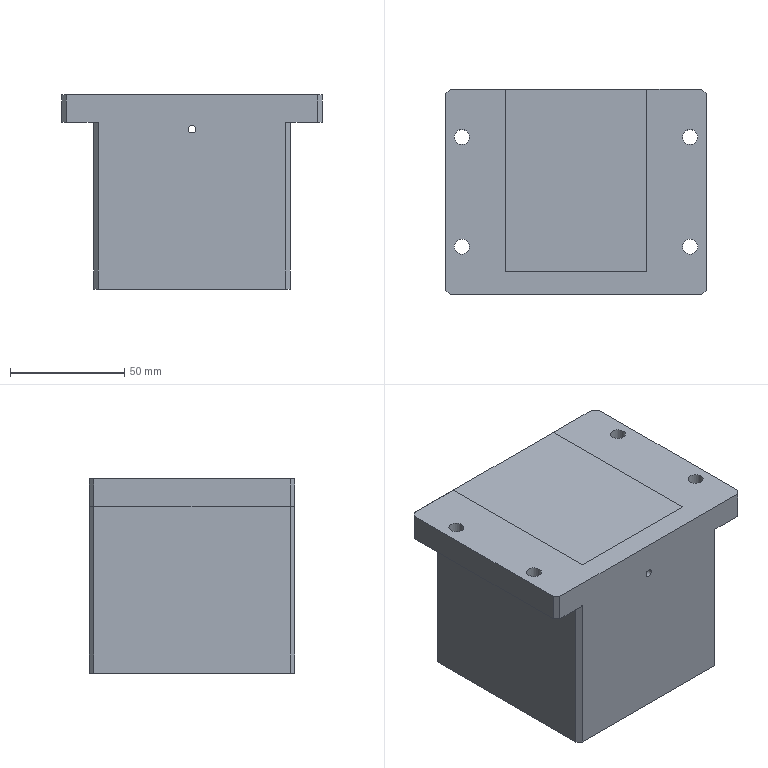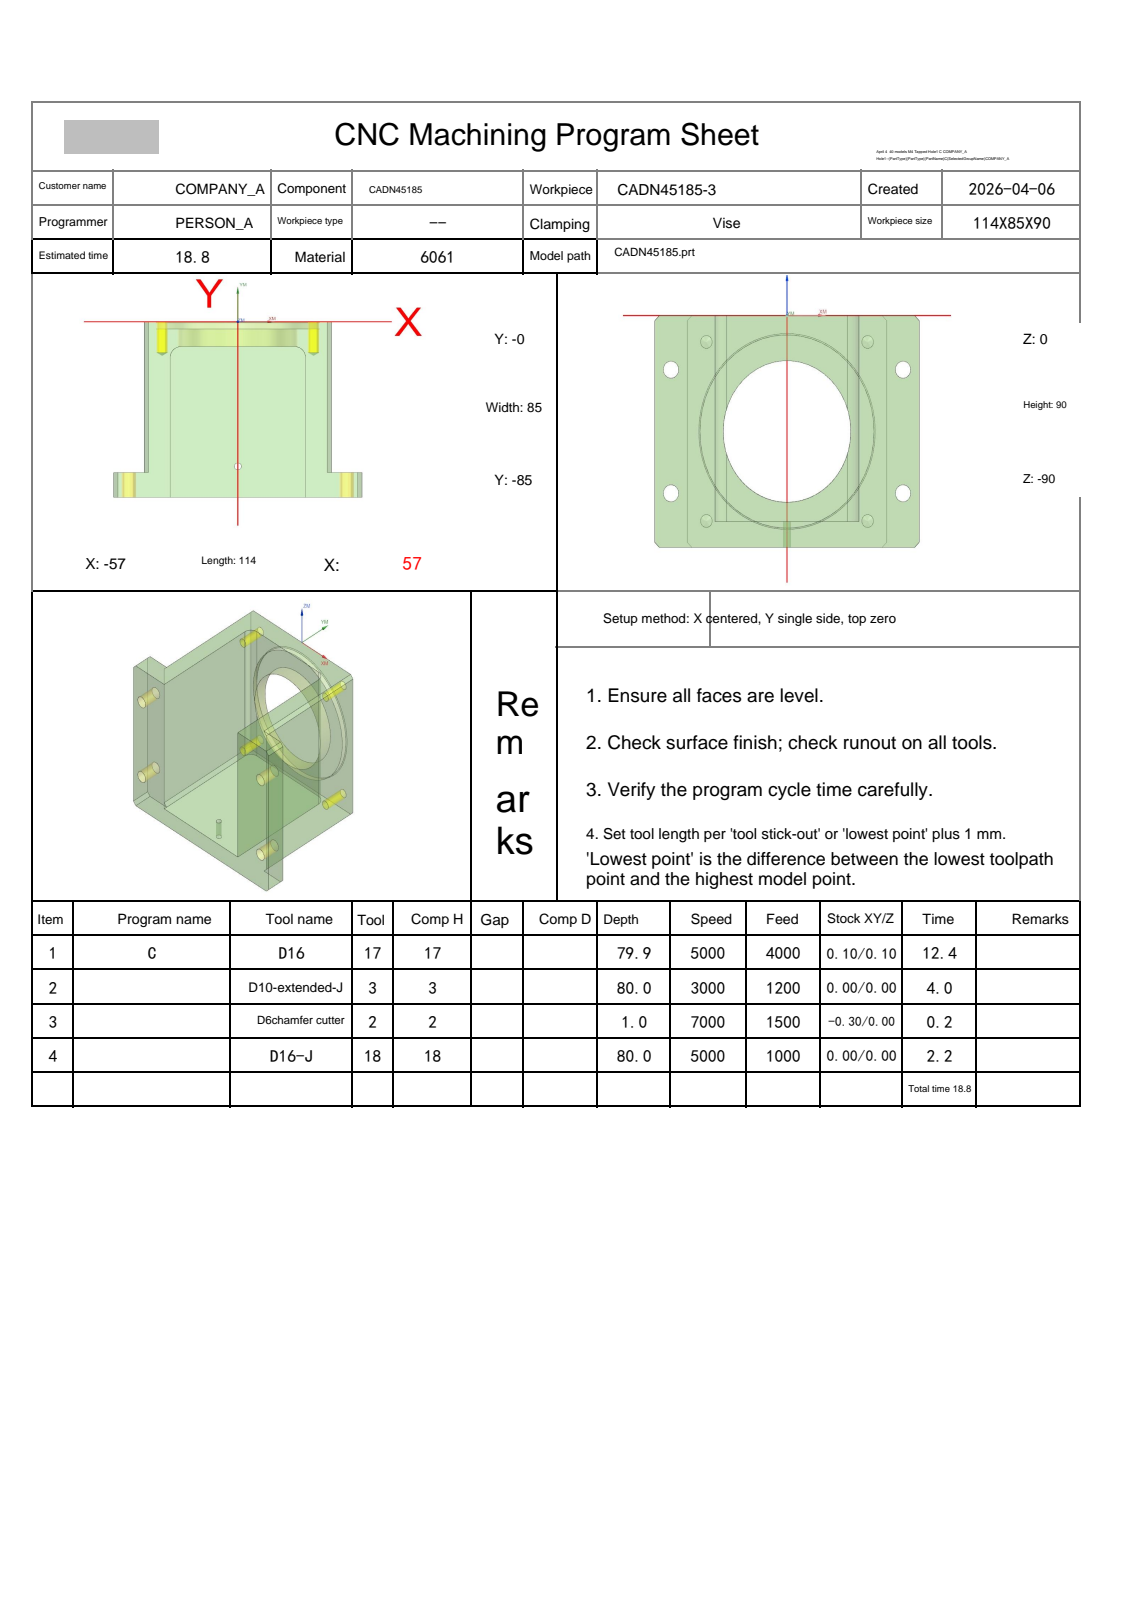NC program | NX | posted by the shop | part box 114 x 90 x 85 mm
Lines 1 to 1245 of 14367:
%
O0001
(Machine time: 19.44 MIN)
(===Total Tool:4===)
(T17=D16    D=16.  R=0.   D-  H17 Z=-79.9 )
(T3=D10-extended-J D=10.  R=0.   D-  H03 Z=-80.  )
(T2=D6chamfer cutter   D=6.   R=0.   D-  H02 Z=-1.   )
(T18=D16-J  D=16.  R=0.   D18 H18 Z=-80.  )
G80 G90 G17 G49 G40
G91 G28 Z0
M01
N1 T17 M06
(D16  D=16. R=0. H=17 ce=0.10 di=0.10)
G00 G90 G54 X3.936 Y-96. M03 S5000
G43 H17 Z10.1
M08
Z.701
G01 Z-.799 F4000.
X4.104 Y-92.84
X7.098 Y-36.478
G03 X7.104 Y-36.265 I-3.994 J.212
X3.104 Y-32.265 I-4. J0.0
X-.891 Y-36.053 I0.0 J-4.
G01 X-3.827 Y-91.325
G02 X-5.425 Y-92.84 I-1.598 J.085
G01 X-9.3
G02 X-10.9 Y-91.24 I0.0 J1.6
G01 Y-33.697
G02 X-9.303 Y-32.1 I1.6 J-.003
G01 X9.303
G02 X10.9 Y-33.697 I-.003 J-1.6
G01 Y-91.471
G03 X12.253 Y-93.051 I1.6 J.001
G01 X21.054 Y-94.421
G03 X21.3 Y-94.44 I.246 J1.581
X22.9 Y-92.84 I0.0 J1.6
G01 Y-20.1
X-22.9
Y-92.84
Y-96.1
Z.701
G00 X3.936 Y-96.
Z-.098
G01 Z-1.598
X4.104 Y-92.84
X7.098 Y-36.478
G03 X7.104 Y-36.265 I-3.994 J.212
X3.104 Y-32.265 I-4. J0.0
X-.891 Y-36.053 I0.0 J-4.
G01 X-3.827 Y-91.325
G02 X-5.425 Y-92.84 I-1.598 J.085
G01 X-9.3
G02 X-10.9 Y-91.24 I0.0 J1.6
G01 Y-33.697
G02 X-9.303 Y-32.1 I1.6 J-.003
G01 X9.303
G02 X10.9 Y-33.697 I-.003 J-1.6
G01 Y-91.471
G03 X12.253 Y-93.051 I1.6 J.001
G01 X21.054 Y-94.421
G03 X21.3 Y-94.44 I.246 J1.581
X22.9 Y-92.84 I0.0 J1.6
G01 Y-20.1
X-22.9
Y-92.84
Y-96.1
Z-.098
G00 X3.936 Y-96.
Z-.897
G01 Z-2.397
X4.104 Y-92.84
X7.098 Y-36.478
G03 X7.104 Y-36.265 I-3.994 J.212
X3.104 Y-32.265 I-4. J0.0
X-.891 Y-36.053 I0.0 J-4.
G01 X-3.827 Y-91.325
G02 X-5.425 Y-92.84 I-1.598 J.085
G01 X-9.3
G02 X-10.9 Y-91.24 I0.0 J1.6
G01 Y-33.697
G02 X-9.303 Y-32.1 I1.6 J-.003
G01 X9.303
G02 X10.9 Y-33.697 I-.003 J-1.6
G01 Y-91.471
G03 X12.253 Y-93.051 I1.6 J.001
G01 X21.054 Y-94.421
G03 X21.3 Y-94.44 I.246 J1.581
X22.9 Y-92.84 I0.0 J1.6
G01 Y-20.1
X-22.9
Y-92.84
Y-96.1
Z-.897
G00 X3.936 Y-96.
Z-1.696
G01 Z-3.196
X4.104 Y-92.84
X7.098 Y-36.478
G03 X7.104 Y-36.265 I-3.994 J.212
X3.104 Y-32.265 I-4. J0.0
X-.891 Y-36.053 I0.0 J-4.
G01 X-3.827 Y-91.325
G02 X-5.425 Y-92.84 I-1.598 J.085
G01 X-9.3
G02 X-10.9 Y-91.24 I0.0 J1.6
G01 Y-33.697
G02 X-9.303 Y-32.1 I1.6 J-.003
G01 X9.303
G02 X10.9 Y-33.697 I-.003 J-1.6
G01 Y-91.471
G03 X12.253 Y-93.051 I1.6 J.001
G01 X21.054 Y-94.421
G03 X21.3 Y-94.44 I.246 J1.581
X22.9 Y-92.84 I0.0 J1.6
G01 Y-20.1
X-22.9
Y-92.84
Y-96.1
Z-1.696
G00 X3.936 Y-96.
Z-2.495
G01 Z-3.995
X4.104 Y-92.84
X7.098 Y-36.478
G03 X7.104 Y-36.265 I-3.994 J.212
X3.104 Y-32.265 I-4. J0.0
X-.891 Y-36.053 I0.0 J-4.
G01 X-3.827 Y-91.325
G02 X-5.425 Y-92.84 I-1.598 J.085
G01 X-9.3
G02 X-10.9 Y-91.24 I0.0 J1.6
G01 Y-33.697
G02 X-9.303 Y-32.1 I1.6 J-.003
G01 X9.303
G02 X10.9 Y-33.697 I-.003 J-1.6
G01 Y-91.471
G03 X12.253 Y-93.051 I1.6 J.001
G01 X21.054 Y-94.421
G03 X21.3 Y-94.44 I.246 J1.581
X22.9 Y-92.84 I0.0 J1.6
G01 Y-20.1
X-22.9
Y-92.84
Y-96.1
Z-2.495
G00 X3.936 Y-96.
Z-3.294
G01 Z-4.794
X4.104 Y-92.84
X7.098 Y-36.478
G03 X7.104 Y-36.265 I-3.994 J.212
X3.104 Y-32.265 I-4. J0.0
X-.891 Y-36.053 I0.0 J-4.
G01 X-3.827 Y-91.325
G02 X-5.425 Y-92.84 I-1.598 J.085
G01 X-9.3
G02 X-10.9 Y-91.24 I0.0 J1.6
G01 Y-33.697
G02 X-9.303 Y-32.1 I1.6 J-.003
G01 X9.303
G02 X10.9 Y-33.697 I-.003 J-1.6
G01 Y-91.471
G03 X12.253 Y-93.051 I1.6 J.001
G01 X21.054 Y-94.421
G03 X21.3 Y-94.44 I.246 J1.581
X22.9 Y-92.84 I0.0 J1.6
G01 Y-20.1
X-22.9
Y-92.84
Y-96.1
Z-3.294
G00 X3.936 Y-96.
Z-4.093
G01 Z-5.593
X4.104 Y-92.84
X7.098 Y-36.478
G03 X7.104 Y-36.265 I-3.994 J.212
X3.104 Y-32.265 I-4. J0.0
X-.891 Y-36.053 I0.0 J-4.
G01 X-3.827 Y-91.325
G02 X-5.425 Y-92.84 I-1.598 J.085
G01 X-9.3
G02 X-10.9 Y-91.24 I0.0 J1.6
G01 Y-33.697
G02 X-9.303 Y-32.1 I1.6 J-.003
G01 X9.303
G02 X10.9 Y-33.697 I-.003 J-1.6
G01 Y-91.471
G03 X12.253 Y-93.051 I1.6 J.001
G01 X21.054 Y-94.421
G03 X21.3 Y-94.44 I.246 J1.581
X22.9 Y-92.84 I0.0 J1.6
G01 Y-20.1
X-22.9
Y-92.84
Y-96.1
Z-4.093
G00 X3.936 Y-96.
Z-4.892
G01 Z-6.392
X4.104 Y-92.84
X7.098 Y-36.478
G03 X7.104 Y-36.265 I-3.994 J.212
X3.104 Y-32.265 I-4. J0.0
X-.891 Y-36.053 I0.0 J-4.
G01 X-3.827 Y-91.325
G02 X-5.425 Y-92.84 I-1.598 J.085
G01 X-9.3
G02 X-10.9 Y-91.24 I0.0 J1.6
G01 Y-33.697
G02 X-9.303 Y-32.1 I1.6 J-.003
G01 X9.303
G02 X10.9 Y-33.697 I-.003 J-1.6
G01 Y-91.471
G03 X12.253 Y-93.051 I1.6 J.001
G01 X21.054 Y-94.421
G03 X21.3 Y-94.44 I.246 J1.581
X22.9 Y-92.84 I0.0 J1.6
G01 Y-20.1
X-22.9
Y-92.84
Y-96.1
Z-4.892
G00 X3.936 Y-96.
Z-5.691
G01 Z-7.191
X4.104 Y-92.84
X7.098 Y-36.478
G03 X7.104 Y-36.265 I-3.994 J.212
X3.104 Y-32.265 I-4. J0.0
X-.891 Y-36.053 I0.0 J-4.
G01 X-3.827 Y-91.325
G02 X-5.425 Y-92.84 I-1.598 J.085
G01 X-9.3
G02 X-10.9 Y-91.24 I0.0 J1.6
G01 Y-33.697
G02 X-9.303 Y-32.1 I1.6 J-.003
G01 X9.303
G02 X10.9 Y-33.697 I-.003 J-1.6
G01 Y-91.471
G03 X12.253 Y-93.051 I1.6 J.001
G01 X21.054 Y-94.421
G03 X21.3 Y-94.44 I.246 J1.581
X22.9 Y-92.84 I0.0 J1.6
G01 Y-20.1
X-22.9
Y-92.84
Y-96.1
Z-5.691
G00 X3.936 Y-96.
Z-6.49
G01 Z-7.99
X4.104 Y-92.84
X7.098 Y-36.478
G03 X7.104 Y-36.265 I-3.994 J.212
X3.104 Y-32.265 I-4. J0.0
X-.891 Y-36.053 I0.0 J-4.
G01 X-3.827 Y-91.325
G02 X-5.425 Y-92.84 I-1.598 J.085
G01 X-9.3
G02 X-10.9 Y-91.24 I0.0 J1.6
G01 Y-33.697
G02 X-9.303 Y-32.1 I1.6 J-.003
G01 X9.303
G02 X10.9 Y-33.697 I-.003 J-1.6
G01 Y-91.471
G03 X12.253 Y-93.051 I1.6 J.001
G01 X21.054 Y-94.421
G03 X21.3 Y-94.44 I.246 J1.581
X22.9 Y-92.84 I0.0 J1.6
G01 Y-20.1
X-22.9
Y-92.84
Y-96.1
Z-6.49
G00 X3.936 Y-96.
Z-7.289
G01 Z-8.789
X4.104 Y-92.84
X7.098 Y-36.478
G03 X7.104 Y-36.265 I-3.994 J.212
X3.104 Y-32.265 I-4. J0.0
X-.891 Y-36.053 I0.0 J-4.
G01 X-3.827 Y-91.325
G02 X-5.425 Y-92.84 I-1.598 J.085
G01 X-9.3
G02 X-10.9 Y-91.24 I0.0 J1.6
G01 Y-33.697
G02 X-9.303 Y-32.1 I1.6 J-.003
G01 X9.303
G02 X10.9 Y-33.697 I-.003 J-1.6
G01 Y-91.471
G03 X12.253 Y-93.051 I1.6 J.001
G01 X21.054 Y-94.421
G03 X21.3 Y-94.44 I.246 J1.581
X22.9 Y-92.84 I0.0 J1.6
G01 Y-20.1
X-22.9
Y-92.84
Y-96.1
Z-7.289
G00 X3.936 Y-96.
Z-8.088
G01 Z-9.588
X4.104 Y-92.84
X7.098 Y-36.478
G03 X7.104 Y-36.265 I-3.994 J.212
X3.104 Y-32.265 I-4. J0.0
X-.891 Y-36.053 I0.0 J-4.
G01 X-3.827 Y-91.325
G02 X-5.425 Y-92.84 I-1.598 J.085
G01 X-9.3
G02 X-10.9 Y-91.24 I0.0 J1.6
G01 Y-33.697
G02 X-9.303 Y-32.1 I1.6 J-.003
G01 X9.303
G02 X10.9 Y-33.697 I-.003 J-1.6
G01 Y-91.471
G03 X12.253 Y-93.051 I1.6 J.001
G01 X21.054 Y-94.421
G03 X21.3 Y-94.44 I.246 J1.581
X22.9 Y-92.84 I0.0 J1.6
G01 Y-20.1
X-22.9
Y-92.84
Y-96.1
Z-8.088
G00 X3.936 Y-96.
Z-8.887
G01 Z-10.387
X4.104 Y-92.84
X7.098 Y-36.478
G03 X7.104 Y-36.265 I-3.994 J.212
X3.104 Y-32.265 I-4. J0.0
X-.891 Y-36.053 I0.0 J-4.
G01 X-3.827 Y-91.325
G02 X-5.425 Y-92.84 I-1.598 J.085
G01 X-9.3
G02 X-10.9 Y-91.24 I0.0 J1.6
G01 Y-33.697
G02 X-9.303 Y-32.1 I1.6 J-.003
G01 X9.303
G02 X10.9 Y-33.697 I-.003 J-1.6
G01 Y-91.471
G03 X12.253 Y-93.051 I1.6 J.001
G01 X21.054 Y-94.421
G03 X21.3 Y-94.44 I.246 J1.581
X22.9 Y-92.84 I0.0 J1.6
G01 Y-20.1
X-22.9
Y-92.84
Y-96.1
Z-8.887
G00 X3.936 Y-96.
Z-9.686
G01 Z-11.186
X4.104 Y-92.84
X7.098 Y-36.478
G03 X7.104 Y-36.265 I-3.994 J.212
X3.104 Y-32.265 I-4. J0.0
X-.891 Y-36.053 I0.0 J-4.
G01 X-3.827 Y-91.325
G02 X-5.425 Y-92.84 I-1.598 J.085
G01 X-9.3
G02 X-10.9 Y-91.24 I0.0 J1.6
G01 Y-33.697
G02 X-9.303 Y-32.1 I1.6 J-.003
G01 X9.303
G02 X10.9 Y-33.697 I-.003 J-1.6
G01 Y-91.471
G03 X12.253 Y-93.051 I1.6 J.001
G01 X21.054 Y-94.421
G03 X21.3 Y-94.44 I.246 J1.581
X22.9 Y-92.84 I0.0 J1.6
G01 Y-20.1
X-22.9
Y-92.84
Y-96.1
Z-9.686
G00 X3.936 Y-96.
Z-10.485
G01 Z-11.985
X4.104 Y-92.84
X7.098 Y-36.478
G03 X7.104 Y-36.265 I-3.994 J.212
X3.104 Y-32.265 I-4. J0.0
X-.891 Y-36.053 I0.0 J-4.
G01 X-3.827 Y-91.325
G02 X-5.425 Y-92.84 I-1.598 J.085
G01 X-9.3
G02 X-10.9 Y-91.24 I0.0 J1.6
G01 Y-33.697
G02 X-9.303 Y-32.1 I1.6 J-.003
G01 X9.303
G02 X10.9 Y-33.697 I-.003 J-1.6
G01 Y-91.471
G03 X12.253 Y-93.051 I1.6 J.001
G01 X21.054 Y-94.421
G03 X21.3 Y-94.44 I.246 J1.581
X22.9 Y-92.84 I0.0 J1.6
G01 Y-20.1
X-22.9
Y-92.84
Y-96.1
Z-10.485
G00 X3.936 Y-96.
Z-11.284
G01 Z-12.784
X4.104 Y-92.84
X7.098 Y-36.478
G03 X7.104 Y-36.265 I-3.994 J.212
X3.104 Y-32.265 I-4. J0.0
X-.891 Y-36.053 I0.0 J-4.
G01 X-3.827 Y-91.325
G02 X-5.425 Y-92.84 I-1.598 J.085
G01 X-9.3
G02 X-10.9 Y-91.24 I0.0 J1.6
G01 Y-33.697
G02 X-9.303 Y-32.1 I1.6 J-.003
G01 X9.303
G02 X10.9 Y-33.697 I-.003 J-1.6
G01 Y-91.471
G03 X12.253 Y-93.051 I1.6 J.001
G01 X21.054 Y-94.421
G03 X21.3 Y-94.44 I.246 J1.581
X22.9 Y-92.84 I0.0 J1.6
G01 Y-20.1
X-22.9
Y-92.84
Y-96.1
Z-11.284
G00 X3.936 Y-96.
Z-12.083
G01 Z-13.583
X4.104 Y-92.84
X7.098 Y-36.478
G03 X7.104 Y-36.265 I-3.994 J.212
X3.104 Y-32.265 I-4. J0.0
X-.891 Y-36.053 I0.0 J-4.
G01 X-3.827 Y-91.325
G02 X-5.425 Y-92.84 I-1.598 J.085
G01 X-9.3
G02 X-10.9 Y-91.24 I0.0 J1.6
G01 Y-33.697
G02 X-9.303 Y-32.1 I1.6 J-.003
G01 X9.303
G02 X10.9 Y-33.697 I-.003 J-1.6
G01 Y-91.471
G03 X12.253 Y-93.051 I1.6 J.001
G01 X21.054 Y-94.421
G03 X21.3 Y-94.44 I.246 J1.581
X22.9 Y-92.84 I0.0 J1.6
G01 Y-20.1
X-22.9
Y-92.84
Y-96.1
Z-12.083
G00 X3.936 Y-96.
Z-12.882
G01 Z-14.382
X4.104 Y-92.84
X7.098 Y-36.478
G03 X7.104 Y-36.265 I-3.994 J.212
X3.104 Y-32.265 I-4. J0.0
X-.891 Y-36.053 I0.0 J-4.
G01 X-3.827 Y-91.325
G02 X-5.425 Y-92.84 I-1.598 J.085
G01 X-9.3
G02 X-10.9 Y-91.24 I0.0 J1.6
G01 Y-33.697
G02 X-9.303 Y-32.1 I1.6 J-.003
G01 X9.303
G02 X10.9 Y-33.697 I-.003 J-1.6
G01 Y-91.471
G03 X12.253 Y-93.051 I1.6 J.001
G01 X21.054 Y-94.421
G03 X21.3 Y-94.44 I.246 J1.581
X22.9 Y-92.84 I0.0 J1.6
G01 Y-20.1
X-22.9
Y-92.84
Y-96.1
Z-12.882
G00 X3.936 Y-96.
Z-13.681
G01 Z-15.181
X4.104 Y-92.84
X7.098 Y-36.478
G03 X7.104 Y-36.265 I-3.994 J.212
X3.104 Y-32.265 I-4. J0.0
X-.891 Y-36.053 I0.0 J-4.
G01 X-3.827 Y-91.325
G02 X-5.425 Y-92.84 I-1.598 J.085
G01 X-9.3
G02 X-10.9 Y-91.24 I0.0 J1.6
G01 Y-33.697
G02 X-9.303 Y-32.1 I1.6 J-.003
G01 X9.303
G02 X10.9 Y-33.697 I-.003 J-1.6
G01 Y-91.471
G03 X12.253 Y-93.051 I1.6 J.001
G01 X21.054 Y-94.421
G03 X21.3 Y-94.44 I.246 J1.581
X22.9 Y-92.84 I0.0 J1.6
G01 Y-20.1
X-22.9
Y-92.84
Y-96.1
Z-13.681
G00 X3.936 Y-96.
Z-14.48
G01 Z-15.98
X4.104 Y-92.84
X7.098 Y-36.478
G03 X7.104 Y-36.265 I-3.994 J.212
X3.104 Y-32.265 I-4. J0.0
X-.891 Y-36.053 I0.0 J-4.
G01 X-3.827 Y-91.325
G02 X-5.425 Y-92.84 I-1.598 J.085
G01 X-9.3
G02 X-10.9 Y-91.24 I0.0 J1.6
G01 Y-33.697
G02 X-9.303 Y-32.1 I1.6 J-.003
G01 X9.303
G02 X10.9 Y-33.697 I-.003 J-1.6
G01 Y-91.471
G03 X12.253 Y-93.051 I1.6 J.001
G01 X21.054 Y-94.421
G03 X21.3 Y-94.44 I.246 J1.581
X22.9 Y-92.84 I0.0 J1.6
G01 Y-20.1
X-22.9
Y-92.84
Y-96.1
Z-14.48
G00 X3.936 Y-96.
Z-15.279
G01 Z-16.779
X4.104 Y-92.84
X7.098 Y-36.478
G03 X7.104 Y-36.265 I-3.994 J.212
X3.104 Y-32.265 I-4. J0.0
X-.891 Y-36.053 I0.0 J-4.
G01 X-3.827 Y-91.325
G02 X-5.425 Y-92.84 I-1.598 J.085
G01 X-9.3
G02 X-10.9 Y-91.24 I0.0 J1.6
G01 Y-33.697
G02 X-9.303 Y-32.1 I1.6 J-.003
G01 X9.303
G02 X10.9 Y-33.697 I-.003 J-1.6
G01 Y-91.471
G03 X12.253 Y-93.051 I1.6 J.001
G01 X21.054 Y-94.421
G03 X21.3 Y-94.44 I.246 J1.581
X22.9 Y-92.84 I0.0 J1.6
G01 Y-20.1
X-22.9
Y-92.84
Y-96.1
Z-15.279
G00 X3.936 Y-96.
Z-16.078
G01 Z-17.578
X4.104 Y-92.84
X7.098 Y-36.478
G03 X7.104 Y-36.265 I-3.994 J.212
X3.104 Y-32.265 I-4. J0.0
X-.891 Y-36.053 I0.0 J-4.
G01 X-3.827 Y-91.325
G02 X-5.425 Y-92.84 I-1.598 J.085
G01 X-9.3
G02 X-10.9 Y-91.24 I0.0 J1.6
G01 Y-33.697
G02 X-9.303 Y-32.1 I1.6 J-.003
G01 X9.303
G02 X10.9 Y-33.697 I-.003 J-1.6
G01 Y-91.471
G03 X12.253 Y-93.051 I1.6 J.001
G01 X21.054 Y-94.421
G03 X21.3 Y-94.44 I.246 J1.581
X22.9 Y-92.84 I0.0 J1.6
G01 Y-20.1
X-22.9
Y-92.84
Y-96.1
Z-16.078
G00 X3.936 Y-96.
Z-16.877
G01 Z-18.377
X4.104 Y-92.84
X7.098 Y-36.478
G03 X7.104 Y-36.265 I-3.994 J.212
X3.104 Y-32.265 I-4. J0.0
X-.891 Y-36.053 I0.0 J-4.
G01 X-3.827 Y-91.325
G02 X-5.425 Y-92.84 I-1.598 J.085
G01 X-9.3
G02 X-10.9 Y-91.24 I0.0 J1.6
G01 Y-33.697
G02 X-9.303 Y-32.1 I1.6 J-.003
G01 X9.303
G02 X10.9 Y-33.697 I-.003 J-1.6
G01 Y-91.471
G03 X12.253 Y-93.051 I1.6 J.001
G01 X21.054 Y-94.421
G03 X21.3 Y-94.44 I.246 J1.581
X22.9 Y-92.84 I0.0 J1.6
G01 Y-20.1
X-22.9
Y-92.84
Y-96.1
Z-16.877
G00 X3.936 Y-96.
Z-17.676
G01 Z-19.176
X4.104 Y-92.84
X7.098 Y-36.478
G03 X7.104 Y-36.265 I-3.994 J.212
X3.104 Y-32.265 I-4. J0.0
X-.891 Y-36.053 I0.0 J-4.
G01 X-3.827 Y-91.325
G02 X-5.425 Y-92.84 I-1.598 J.085
G01 X-9.3
G02 X-10.9 Y-91.24 I0.0 J1.6
G01 Y-33.697
G02 X-9.303 Y-32.1 I1.6 J-.003
G01 X9.303
G02 X10.9 Y-33.697 I-.003 J-1.6
G01 Y-91.471
G03 X12.253 Y-93.051 I1.6 J.001
G01 X21.054 Y-94.421
G03 X21.3 Y-94.44 I.246 J1.581
X22.9 Y-92.84 I0.0 J1.6
G01 Y-20.1
X-22.9
Y-92.84
Y-96.1
Z-17.676
G00 X3.936 Y-96.
Z-18.475
G01 Z-19.975
X4.104 Y-92.84
X7.098 Y-36.478
G03 X7.104 Y-36.265 I-3.994 J.212
X3.104 Y-32.265 I-4. J0.0
X-.891 Y-36.053 I0.0 J-4.
G01 X-3.827 Y-91.325
G02 X-5.425 Y-92.84 I-1.598 J.085
G01 X-9.3
G02 X-10.9 Y-91.24 I0.0 J1.6
G01 Y-33.697
G02 X-9.303 Y-32.1 I1.6 J-.003
G01 X9.303
G02 X10.9 Y-33.697 I-.003 J-1.6
G01 Y-91.471
G03 X12.253 Y-93.051 I1.6 J.001
G01 X21.054 Y-94.421
G03 X21.3 Y-94.44 I.246 J1.581
X22.9 Y-92.84 I0.0 J1.6
G01 Y-20.1
X-22.9
Y-92.84
Y-96.1
Z-18.475
G00 X3.936 Y-96.
Z-19.274
G01 Z-20.774
X4.104 Y-92.84
X7.098 Y-36.478
G03 X7.104 Y-36.265 I-3.994 J.212
X3.104 Y-32.265 I-4. J0.0
X-.891 Y-36.053 I0.0 J-4.
G01 X-3.827 Y-91.325
G02 X-5.425 Y-92.84 I-1.598 J.085
G01 X-9.3
G02 X-10.9 Y-91.24 I0.0 J1.6
G01 Y-33.697
G02 X-9.303 Y-32.1 I1.6 J-.003
G01 X9.303
G02 X10.9 Y-33.697 I-.003 J-1.6
G01 Y-91.471
G03 X12.253 Y-93.051 I1.6 J.001
G01 X21.054 Y-94.421
G03 X21.3 Y-94.44 I.246 J1.581
X22.9 Y-92.84 I0.0 J1.6
G01 Y-20.1
X-22.9
Y-92.84
Y-96.1
Z-19.274
G00 X3.936 Y-96.
Z-20.073
G01 Z-21.573
X4.104 Y-92.84
X7.098 Y-36.478
G03 X7.104 Y-36.265 I-3.994 J.212
X3.104 Y-32.265 I-4. J0.0
X-.891 Y-36.053 I0.0 J-4.
G01 X-3.827 Y-91.325
G02 X-5.425 Y-92.84 I-1.598 J.085
G01 X-9.3
G02 X-10.9 Y-91.24 I0.0 J1.6
G01 Y-33.697
G02 X-9.303 Y-32.1 I1.6 J-.003
G01 X9.303
G02 X10.9 Y-33.697 I-.003 J-1.6
G01 Y-91.471
G03 X12.253 Y-93.051 I1.6 J.001
G01 X21.054 Y-94.421
G03 X21.3 Y-94.44 I.246 J1.581
X22.9 Y-92.84 I0.0 J1.6
G01 Y-20.1
X-22.9
Y-92.84
Y-96.1
Z-20.073
G00 X3.936 Y-96.
Z-20.872
G01 Z-22.372
X4.104 Y-92.84
X7.098 Y-36.478
G03 X7.104 Y-36.265 I-3.994 J.212
X3.104 Y-32.265 I-4. J0.0
X-.891 Y-36.053 I0.0 J-4.
G01 X-3.827 Y-91.325
G02 X-5.425 Y-92.84 I-1.598 J.085
G01 X-9.3
G02 X-10.9 Y-91.24 I0.0 J1.6
G01 Y-33.697
G02 X-9.303 Y-32.1 I1.6 J-.003
G01 X9.303
G02 X10.9 Y-33.697 I-.003 J-1.6
G01 Y-91.471
G03 X12.253 Y-93.051 I1.6 J.001
G01 X21.054 Y-94.421
G03 X21.3 Y-94.44 I.246 J1.581
X22.9 Y-92.84 I0.0 J1.6
G01 Y-20.1
X-22.9
Y-92.84
Y-96.1
Z-20.872
G00 X3.936 Y-96.
Z-21.671
G01 Z-23.171
X4.104 Y-92.84
X7.098 Y-36.478
G03 X7.104 Y-36.265 I-3.994 J.212
X3.104 Y-32.265 I-4. J0.0
X-.891 Y-36.053 I0.0 J-4.
G01 X-3.827 Y-91.325
G02 X-5.425 Y-92.84 I-1.598 J.085
G01 X-9.3
G02 X-10.9 Y-91.24 I0.0 J1.6
G01 Y-33.697
G02 X-9.303 Y-32.1 I1.6 J-.003
G01 X9.303
G02 X10.9 Y-33.697 I-.003 J-1.6
G01 Y-91.471
G03 X12.253 Y-93.051 I1.6 J.001
G01 X21.054 Y-94.421
G03 X21.3 Y-94.44 I.246 J1.581
X22.9 Y-92.84 I0.0 J1.6
G01 Y-20.1
X-22.9
Y-92.84
Y-96.1
Z-21.671
G00 X3.936 Y-96.
Z-22.47
G01 Z-23.97
X4.104 Y-92.84
X7.098 Y-36.478
G03 X7.104 Y-36.265 I-3.994 J.212
X3.104 Y-32.265 I-4. J0.0
X-.891 Y-36.053 I0.0 J-4.
G01 X-3.827 Y-91.325
G02 X-5.425 Y-92.84 I-1.598 J.085
G01 X-9.3
G02 X-10.9 Y-91.24 I0.0 J1.6
G01 Y-33.697
G02 X-9.303 Y-32.1 I1.6 J-.003
G01 X9.303
G02 X10.9 Y-33.697 I-.003 J-1.6
G01 Y-91.471
G03 X12.253 Y-93.051 I1.6 J.001
G01 X21.054 Y-94.421
G03 X21.3 Y-94.44 I.246 J1.581
X22.9 Y-92.84 I0.0 J1.6
G01 Y-20.1
X-22.9
Y-92.84
Y-96.1
Z-22.47
G00 X3.936 Y-96.
Z-23.269
G01 Z-24.769
X4.104 Y-92.84
X7.098 Y-36.478
G03 X7.104 Y-36.265 I-3.994 J.212
X3.104 Y-32.265 I-4. J0.0
X-.891 Y-36.053 I0.0 J-4.
G01 X-3.827 Y-91.325
G02 X-5.425 Y-92.84 I-1.598 J.085
G01 X-9.3
G02 X-10.9 Y-91.24 I0.0 J1.6
G01 Y-33.697
G02 X-9.303 Y-32.1 I1.6 J-.003
G01 X9.303
G02 X10.9 Y-33.697 I-.003 J-1.6
G01 Y-91.471
G03 X12.253 Y-93.051 I1.6 J.001
G01 X21.054 Y-94.421
G03 X21.3 Y-94.44 I.246 J1.581
X22.9 Y-92.84 I0.0 J1.6
G01 Y-20.1
X-22.9
Y-92.84
Y-96.1
Z-23.269
G00 X3.936 Y-96.
Z-24.068
G01 Z-25.568
X4.104 Y-92.84
X7.098 Y-36.478
G03 X7.104 Y-36.265 I-3.994 J.212
X3.104 Y-32.265 I-4. J0.0
X-.891 Y-36.053 I0.0 J-4.
G01 X-3.827 Y-91.325
G02 X-5.425 Y-92.84 I-1.598 J.085
G01 X-9.3
G02 X-10.9 Y-91.24 I0.0 J1.6
G01 Y-33.697
G02 X-9.303 Y-32.1 I1.6 J-.003
G01 X9.303
G02 X10.9 Y-33.697 I-.003 J-1.6
G01 Y-91.471
G03 X12.253 Y-93.051 I1.6 J.001
G01 X21.054 Y-94.421
G03 X21.3 Y-94.44 I.246 J1.581
X22.9 Y-92.84 I0.0 J1.6
G01 Y-20.1
X-22.9
Y-92.84
Y-96.1
Z-24.068
G00 X3.936 Y-96.
Z-24.867
G01 Z-26.367
X4.104 Y-92.84
X7.098 Y-36.478
G03 X7.104 Y-36.265 I-3.994 J.212
X3.104 Y-32.265 I-4. J0.0
X-.891 Y-36.053 I0.0 J-4.
G01 X-3.827 Y-91.325
G02 X-5.425 Y-92.84 I-1.598 J.085
G01 X-9.3
G02 X-10.9 Y-91.24 I0.0 J1.6
G01 Y-33.697
G02 X-9.303 Y-32.1 I1.6 J-.003
G01 X9.303
G02 X10.9 Y-33.697 I-.003 J-1.6
G01 Y-91.471
G03 X12.253 Y-93.051 I1.6 J.001
G01 X21.054 Y-94.421
G03 X21.3 Y-94.44 I.246 J1.581
X22.9 Y-92.84 I0.0 J1.6
G01 Y-20.1
X-22.9
Y-92.84
Y-96.1
Z-24.867
G00 X3.936 Y-96.
Z-25.666
G01 Z-27.166
X4.104 Y-92.84
X7.098 Y-36.478
G03 X7.104 Y-36.265 I-3.994 J.212
X3.104 Y-32.265 I-4. J0.0
X-.891 Y-36.053 I0.0 J-4.
G01 X-3.827 Y-91.325
G02 X-5.425 Y-92.84 I-1.598 J.085
G01 X-9.3
G02 X-10.9 Y-91.24 I0.0 J1.6
G01 Y-33.697
G02 X-9.303 Y-32.1 I1.6 J-.003
G01 X9.303
G02 X10.9 Y-33.697 I-.003 J-1.6
G01 Y-91.471
G03 X12.253 Y-93.051 I1.6 J.001
G01 X21.054 Y-94.421
G03 X21.3 Y-94.44 I.246 J1.581
X22.9 Y-92.84 I0.0 J1.6
G01 Y-20.1
X-22.9
Y-92.84
Y-96.1
Z-25.666
G00 X3.936 Y-96.
Z-26.465
G01 Z-27.965
X4.104 Y-92.84
X7.098 Y-36.478
G03 X7.104 Y-36.265 I-3.994 J.212
X3.104 Y-32.265 I-4. J0.0
X-.891 Y-36.053 I0.0 J-4.
G01 X-3.827 Y-91.325
G02 X-5.425 Y-92.84 I-1.598 J.085
G01 X-9.3
G02 X-10.9 Y-91.24 I0.0 J1.6
G01 Y-33.697
G02 X-9.303 Y-32.1 I1.6 J-.003
G01 X9.303
G02 X10.9 Y-33.697 I-.003 J-1.6
G01 Y-91.471
G03 X12.253 Y-93.051 I1.6 J.001
G01 X21.054 Y-94.421
G03 X21.3 Y-94.44 I.246 J1.581
X22.9 Y-92.84 I0.0 J1.6
G01 Y-20.1
X-22.9
Y-92.84
Y-96.1
Z-26.465
G00 X3.936 Y-96.
Z-27.264
G01 Z-28.764
X4.104 Y-92.84
X7.098 Y-36.478
G03 X7.104 Y-36.265 I-3.994 J.212
X3.104 Y-32.265 I-4. J0.0
X-.891 Y-36.053 I0.0 J-4.
G01 X-3.827 Y-91.325
G02 X-5.425 Y-92.84 I-1.598 J.085
G01 X-9.3
G02 X-10.9 Y-91.24 I0.0 J1.6
G01 Y-33.697
G02 X-9.303 Y-32.1 I1.6 J-.003
G01 X9.303
G02 X10.9 Y-33.697 I-.003 J-1.6
G01 Y-91.471
G03 X12.253 Y-93.051 I1.6 J.001
G01 X21.054 Y-94.421
G03 X21.3 Y-94.44 I.246 J1.581
X22.9 Y-92.84 I0.0 J1.6
G01 Y-20.1
X-22.9
Y-92.84
Y-96.1
Z-27.264
G00 X3.936 Y-96.
Z-28.063
G01 Z-29.563
X4.104 Y-92.84
X7.098 Y-36.478
G03 X7.104 Y-36.265 I-3.994 J.212
X3.104 Y-32.265 I-4. J0.0
X-.891 Y-36.053 I0.0 J-4.
G01 X-3.827 Y-91.325
G02 X-5.425 Y-92.84 I-1.598 J.085
G01 X-9.3
G02 X-10.9 Y-91.24 I0.0 J1.6
G01 Y-33.697
G02 X-9.303 Y-32.1 I1.6 J-.003
G01 X9.303
G02 X10.9 Y-33.697 I-.003 J-1.6
G01 Y-91.471
G03 X12.253 Y-93.051 I1.6 J.001
G01 X21.054 Y-94.421
G03 X21.3 Y-94.44 I.246 J1.581
X22.9 Y-92.84 I0.0 J1.6
G01 Y-20.1
X-22.9
Y-92.84
Y-96.1
Z-28.063
G00 X3.936 Y-96.
Z-28.862
G01 Z-30.362
X4.104 Y-92.84
X7.098 Y-36.478
G03 X7.104 Y-36.265 I-3.994 J.212
X3.104 Y-32.265 I-4. J0.0
X-.891 Y-36.053 I0.0 J-4.
G01 X-3.827 Y-91.325
G02 X-5.425 Y-92.84 I-1.598 J.085
G01 X-9.3
G02 X-10.9 Y-91.24 I0.0 J1.6
G01 Y-33.697
G02 X-9.303 Y-32.1 I1.6 J-.003
G01 X9.303
G02 X10.9 Y-33.697 I-.003 J-1.6
G01 Y-91.471
G03 X12.253 Y-93.051 I1.6 J.001
G01 X21.054 Y-94.421
G03 X21.3 Y-94.44 I.246 J1.581
X22.9 Y-92.84 I0.0 J1.6
G01 Y-20.1
X-22.9
Y-92.84
Y-96.1
Z-28.862
G00 X3.936 Y-96.
Z-29.661
G01 Z-31.161
X4.104 Y-92.84
X7.098 Y-36.478
G03 X7.104 Y-36.265 I-3.994 J.212
X3.104 Y-32.265 I-4. J0.0
X-.891 Y-36.053 I0.0 J-4.
G01 X-3.827 Y-91.325
G02 X-5.425 Y-92.84 I-1.598 J.085
G01 X-9.3
G02 X-10.9 Y-91.24 I0.0 J1.6
G01 Y-33.697
G02 X-9.303 Y-32.1 I1.6 J-.003
G01 X9.303
G02 X10.9 Y-33.697 I-.003 J-1.6
G01 Y-91.471
G03 X12.253 Y-93.051 I1.6 J.001
G01 X21.054 Y-94.421
G03 X21.3 Y-94.44 I.246 J1.581
X22.9 Y-92.84 I0.0 J1.6
G01 Y-20.1
X-22.9
Y-92.84
Y-96.1
Z-29.661
G00 X3.936 Y-96.
Z-30.46
G01 Z-31.96
X4.104 Y-92.84
X7.098 Y-36.478
G03 X7.104 Y-36.265 I-3.994 J.212
X3.104 Y-32.265 I-4. J0.0
X-.891 Y-36.053 I0.0 J-4.
G01 X-3.827 Y-91.325
G02 X-5.425 Y-92.84 I-1.598 J.085
G01 X-9.3
G02 X-10.9 Y-91.24 I0.0 J1.6
G01 Y-33.697
G02 X-9.303 Y-32.1 I1.6 J-.003
G01 X9.303
G02 X10.9 Y-33.697 I-.003 J-1.6
G01 Y-91.471
G03 X12.253 Y-93.051 I1.6 J.001
G01 X21.054 Y-94.421
G03 X21.3 Y-94.44 I.246 J1.581
X22.9 Y-92.84 I0.0 J1.6
G01 Y-20.1
X-22.9
Y-92.84
Y-96.1
Z-30.46
G00 X3.936 Y-96.
Z-31.259
G01 Z-32.759
X4.104 Y-92.84
X7.098 Y-36.478
G03 X7.104 Y-36.265 I-3.994 J.212
X3.104 Y-32.265 I-4. J0.0
X-.891 Y-36.053 I0.0 J-4.
G01 X-3.827 Y-91.325
G02 X-5.425 Y-92.84 I-1.598 J.085
G01 X-9.3
G02 X-10.9 Y-91.24 I0.0 J1.6
G01 Y-33.697
G02 X-9.303 Y-32.1 I1.6 J-.003
G01 X9.303
G02 X10.9 Y-33.697 I-.003 J-1.6
G01 Y-91.471
G03 X12.253 Y-93.051 I1.6 J.001
G01 X21.054 Y-94.421
G03 X21.3 Y-94.44 I.246 J1.581
X22.9 Y-92.84 I0.0 J1.6
G01 Y-20.1
X-22.9
Y-92.84
Y-96.1
Z-31.259
G00 X3.936 Y-96.
Z-32.058
G01 Z-33.558
X4.104 Y-92.84
X7.098 Y-36.478
G03 X7.104 Y-36.265 I-3.994 J.212
X3.104 Y-32.265 I-4. J0.0
X-.891 Y-36.053 I0.0 J-4.
G01 X-3.827 Y-91.325
G02 X-5.425 Y-92.84 I-1.598 J.085
G01 X-9.3
G02 X-10.9 Y-91.24 I0.0 J1.6
G01 Y-33.697
G02 X-9.303 Y-32.1 I1.6 J-.003
G01 X9.303
G02 X10.9 Y-33.697 I-.003 J-1.6
G01 Y-91.471
G03 X12.253 Y-93.051 I1.6 J.001
G01 X21.054 Y-94.421
G03 X21.3 Y-94.44 I.246 J1.581
X22.9 Y-92.84 I0.0 J1.6
G01 Y-20.1
X-22.9
Y-92.84
Y-96.1
Z-32.058
G00 X3.936 Y-96.
Z-32.857
G01 Z-34.357
X4.104 Y-92.84
X7.098 Y-36.478
G03 X7.104 Y-36.265 I-3.994 J.212
X3.104 Y-32.265 I-4. J0.0
X-.891 Y-36.053 I0.0 J-4.
G01 X-3.827 Y-91.325
G02 X-5.425 Y-92.84 I-1.598 J.085
G01 X-9.3
G02 X-10.9 Y-91.24 I0.0 J1.6
G01 Y-33.697
G02 X-9.303 Y-32.1 I1.6 J-.003
G01 X9.303
G02 X10.9 Y-33.697 I-.003 J-1.6
G01 Y-91.471
G03 X12.253 Y-93.051 I1.6 J.001
G01 X21.054 Y-94.421
G03 X21.3 Y-94.44 I.246 J1.581
X22.9 Y-92.84 I0.0 J1.6
G01 Y-20.1
X-22.9
Y-92.84
Y-96.1
Z-32.857
G00 X3.936 Y-96.
Z-33.656
G01 Z-35.156
X4.104 Y-92.84
X7.098 Y-36.478
G03 X7.104 Y-36.265 I-3.994 J.212
X3.104 Y-32.265 I-4. J0.0
X-.891 Y-36.053 I0.0 J-4.
G01 X-3.827 Y-91.325
G02 X-5.425 Y-92.84 I-1.598 J.085
G01 X-9.3
G02 X-10.9 Y-91.24 I0.0 J1.6
G01 Y-33.697
G02 X-9.303 Y-32.1 I1.6 J-.003
G01 X9.303
G02 X10.9 Y-33.697 I-.003 J-1.6
G01 Y-91.471
G03 X12.253 Y-93.051 I1.6 J.001
G01 X21.054 Y-94.421
G03 X21.3 Y-94.44 I.246 J1.581
X22.9 Y-92.84 I0.0 J1.6
G01 Y-20.1
X-22.9
Y-92.84
Y-96.1
Z-33.656
G00 X3.936 Y-96.
Z-34.455
G01 Z-35.955
X4.104 Y-92.84
X7.098 Y-36.478
G03 X7.104 Y-36.265 I-3.994 J.212
X3.104 Y-32.265 I-4. J0.0
X-.891 Y-36.053 I0.0 J-4.
G01 X-3.827 Y-91.325
G02 X-5.425 Y-92.84 I-1.598 J.085
G01 X-9.3
G02 X-10.9 Y-91.24 I0.0 J1.6
G01 Y-33.697
G02 X-9.303 Y-32.1 I1.6 J-.003
G01 X9.303
G02 X10.9 Y-33.697 I-.003 J-1.6
G01 Y-91.471
G03 X12.253 Y-93.051 I1.6 J.001
G01 X21.054 Y-94.421
G03 X21.3 Y-94.44 I.246 J1.581
X22.9 Y-92.84 I0.0 J1.6
G01 Y-20.1
X-22.9
Y-92.84
Y-96.1
Z-34.455
G00 X3.936 Y-96.
Z-35.254
G01 Z-36.754
X4.104 Y-92.84
X7.098 Y-36.478
G03 X7.104 Y-36.265 I-3.994 J.212
X3.104 Y-32.265 I-4. J0.0
X-.891 Y-36.053 I0.0 J-4.
G01 X-3.827 Y-91.325
G02 X-5.425 Y-92.84 I-1.598 J.085
G01 X-9.3
G02 X-10.9 Y-91.24 I0.0 J1.6
G01 Y-33.697
G02 X-9.303 Y-32.1 I1.6 J-.003
G01 X9.303
G02 X10.9 Y-33.697 I-.003 J-1.6
G01 Y-91.471
G03 X12.253 Y-93.051 I1.6 J.001
G01 X21.054 Y-94.421
G03 X21.3 Y-94.44 I.246 J1.581
X22.9 Y-92.84 I0.0 J1.6
G01 Y-20.1
X-22.9
Y-92.84
Y-96.1
Z-35.254
G00 X3.936 Y-96.
Z-36.053
G01 Z-37.553
X4.104 Y-92.84
X7.098 Y-36.478
G03 X7.104 Y-36.265 I-3.994 J.212
X3.104 Y-32.265 I-4. J0.0
X-.891 Y-36.053 I0.0 J-4.
G01 X-3.827 Y-91.325
G02 X-5.425 Y-92.84 I-1.598 J.085
G01 X-9.3
G02 X-10.9 Y-91.24 I0.0 J1.6
G01 Y-33.697
G02 X-9.303 Y-32.1 I1.6 J-.003
G01 X9.303
G02 X10.9 Y-33.697 I-.003 J-1.6
G01 Y-91.471
G03 X12.253 Y-93.051 I1.6 J.001
G01 X21.054 Y-94.421
G03 X21.3 Y-94.44 I.246 J1.581
X22.9 Y-92.84 I0.0 J1.6
G01 Y-20.1
X-22.9
Y-92.84
Y-96.1
Z-36.053
G00 X3.936 Y-96.
Z-36.852
G01 Z-38.352
X4.104 Y-92.84
X7.098 Y-36.478
G03 X7.104 Y-36.265 I-3.994 J.212